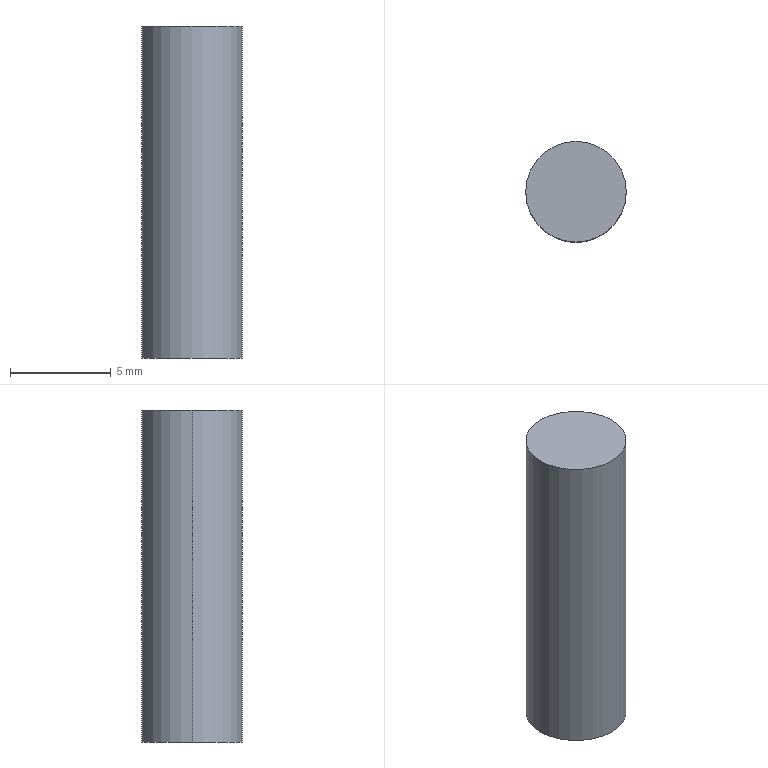Part | STEP file | Top bronze bushing custom screw SGN-2-26 | 1 solid | 11 faces | box 5 x 5 x 16.5 mm | volume 302.577 mm3 | plane 9 | cylinder 2 | commonest cylinder face diameters 5 x2
STEP:
#1=CARTESIAN_POINT('',(0.,0.,0.));
#2=DIRECTION('',(0.,0.,1.));
#3=DIRECTION('',(1.,0.,0.));
#4=AXIS2_PLACEMENT_3D('',#1,#2,#3);
#5=CARTESIAN_POINT('',(2.5,0.,16.5));
#6=VERTEX_POINT('',#5);
#7=CARTESIAN_POINT('',(-2.5,0.,16.5));
#8=VERTEX_POINT('',#7);
#9=CARTESIAN_POINT('',(0.,0.,16.5));
#10=DIRECTION('',(0.,0.,1.));
#11=DIRECTION('',(1.,0.,0.));
#12=AXIS2_PLACEMENT_3D('',#9,#10,#11);
#13=CIRCLE('',#12,2.5);
#14=CARTESIAN_POINT('',(0.,0.,16.5));
#15=DIRECTION('',(0.,0.,-1.));
#16=DIRECTION('',(-1.,0.,0.));
#17=AXIS2_PLACEMENT_3D('',#14,#15,#16);
#18=CYLINDRICAL_SURFACE('',#17,2.5);
#19=CARTESIAN_POINT('',(3.142,0.));
#20=DIRECTION('',(-1.,0.));
#21=VECTOR('',#20,1.);
#22=LINE('',#19,#21);
#23=(GEOMETRIC_REPRESENTATION_CONTEXT(2)PARAMETRIC_REPRESENTATION_CONTEXT()REPRESENTATION_CONTEXT('',''));
#24=DEFINITIONAL_REPRESENTATION('',(#22),#23);
#25=PCURVE('',#18,#24);
#26=CARTESIAN_POINT('',(0.,0.,16.5));
#27=DIRECTION('',(0.,0.,1.));
#28=DIRECTION('',(1.,0.,0.));
#29=AXIS2_PLACEMENT_3D('',#26,#27,#28);
#30=PLANE('',#29);
#31=CARTESIAN_POINT('',(0.,0.));
#32=DIRECTION('',(1.,0.));
#33=AXIS2_PLACEMENT_2D('',#31,#32);
#34=CIRCLE('',#33,2.5);
#35=(GEOMETRIC_REPRESENTATION_CONTEXT(2)PARAMETRIC_REPRESENTATION_CONTEXT()REPRESENTATION_CONTEXT('',''));
#36=DEFINITIONAL_REPRESENTATION('',(#34),#35);
#37=PCURVE('',#30,#36);
#38=SURFACE_CURVE('',#13,(#25,#37),.PCURVE_S1.);
#39=EDGE_CURVE('',#6,#8,#38,.T.);
#40=ORIENTED_EDGE('',*,*,#39,.F.);
#41=CARTESIAN_POINT('',(2.5,0.,0.));
#42=VERTEX_POINT('',#41);
#43=CARTESIAN_POINT('',(2.5,0.,16.5));
#44=DIRECTION('',(0.,0.,-1.));
#45=VECTOR('',#44,1.);
#46=LINE('',#43,#45);
#47=CARTESIAN_POINT('',(3.142,0.));
#48=DIRECTION('',(0.,1.));
#49=VECTOR('',#48,1.);
#50=LINE('',#47,#49);
#51=(GEOMETRIC_REPRESENTATION_CONTEXT(2)PARAMETRIC_REPRESENTATION_CONTEXT()REPRESENTATION_CONTEXT('',''));
#52=DEFINITIONAL_REPRESENTATION('',(#50),#51);
#53=PCURVE('',#18,#52);
#54=CARTESIAN_POINT('',(0.,0.,16.5));
#55=DIRECTION('',(0.,0.,-1.));
#56=DIRECTION('',(-1.,0.,0.));
#57=AXIS2_PLACEMENT_3D('',#54,#55,#56);
#58=CYLINDRICAL_SURFACE('',#57,2.5);
#59=CARTESIAN_POINT('',(3.142,0.));
#60=DIRECTION('',(0.,1.));
#61=VECTOR('',#60,1.);
#62=LINE('',#59,#61);
#63=(GEOMETRIC_REPRESENTATION_CONTEXT(2)PARAMETRIC_REPRESENTATION_CONTEXT()REPRESENTATION_CONTEXT('',''));
#64=DEFINITIONAL_REPRESENTATION('',(#62),#63);
#65=PCURVE('',#58,#64);
#66=SURFACE_CURVE('',#46,(#53,#65),.PCURVE_S1.);
#67=EDGE_CURVE('',#6,#42,#66,.T.);
#68=ORIENTED_EDGE('',*,*,#67,.T.);
#69=CARTESIAN_POINT('',(-2.5,0.,0.));
#70=VERTEX_POINT('',#69);
#71=CARTESIAN_POINT('',(0.,0.,0.));
#72=DIRECTION('',(0.,0.,1.));
#73=DIRECTION('',(1.,0.,0.));
#74=AXIS2_PLACEMENT_3D('',#71,#72,#73);
#75=CIRCLE('',#74,2.5);
#76=CARTESIAN_POINT('',(3.142,16.5));
#77=DIRECTION('',(-1.,0.));
#78=VECTOR('',#77,1.);
#79=LINE('',#76,#78);
#80=(GEOMETRIC_REPRESENTATION_CONTEXT(2)PARAMETRIC_REPRESENTATION_CONTEXT()REPRESENTATION_CONTEXT('',''));
#81=DEFINITIONAL_REPRESENTATION('',(#79),#80);
#82=PCURVE('',#18,#81);
#83=CARTESIAN_POINT('',(0.,0.,0.));
#84=DIRECTION('',(0.,0.,1.));
#85=DIRECTION('',(1.,0.,0.));
#86=AXIS2_PLACEMENT_3D('',#83,#84,#85);
#87=PLANE('',#86);
#88=CARTESIAN_POINT('',(0.,0.));
#89=DIRECTION('',(1.,0.));
#90=AXIS2_PLACEMENT_2D('',#88,#89);
#91=CIRCLE('',#90,2.5);
#92=(GEOMETRIC_REPRESENTATION_CONTEXT(2)PARAMETRIC_REPRESENTATION_CONTEXT()REPRESENTATION_CONTEXT('',''));
#93=DEFINITIONAL_REPRESENTATION('',(#91),#92);
#94=PCURVE('',#87,#93);
#95=SURFACE_CURVE('',#75,(#82,#94),.PCURVE_S1.);
#96=EDGE_CURVE('',#42,#70,#95,.T.);
#97=ORIENTED_EDGE('',*,*,#96,.T.);
#98=CARTESIAN_POINT('',(-2.5,0.,16.5));
#99=DIRECTION('',(0.,0.,-1.));
#100=VECTOR('',#99,1.);
#101=LINE('',#98,#100);
#102=CARTESIAN_POINT('',(0.,0.));
#103=DIRECTION('',(0.,1.));
#104=VECTOR('',#103,1.);
#105=LINE('',#102,#104);
#106=(GEOMETRIC_REPRESENTATION_CONTEXT(2)PARAMETRIC_REPRESENTATION_CONTEXT()REPRESENTATION_CONTEXT('',''));
#107=DEFINITIONAL_REPRESENTATION('',(#105),#106);
#108=PCURVE('',#18,#107);
#109=CARTESIAN_POINT('',(6.283,0.));
#110=DIRECTION('',(0.,1.));
#111=VECTOR('',#110,1.);
#112=LINE('',#109,#111);
#113=(GEOMETRIC_REPRESENTATION_CONTEXT(2)PARAMETRIC_REPRESENTATION_CONTEXT()REPRESENTATION_CONTEXT('',''));
#114=DEFINITIONAL_REPRESENTATION('',(#112),#113);
#115=PCURVE('',#58,#114);
#116=SURFACE_CURVE('',#101,(#108,#115),.PCURVE_S1.);
#117=EDGE_CURVE('',#8,#70,#116,.T.);
#118=ORIENTED_EDGE('',*,*,#117,.F.);
#119=EDGE_LOOP('',(#40,#68,#97,#118));
#120=FACE_BOUND('',#119,.T.);
#121=ADVANCED_FACE('',(#120),#18,.T.);
#122=ORIENTED_EDGE('',*,*,#67,.F.);
#123=CARTESIAN_POINT('',(0.,0.,16.5));
#124=DIRECTION('',(0.,0.,1.));
#125=DIRECTION('',(1.,0.,0.));
#126=AXIS2_PLACEMENT_3D('',#123,#124,#125);
#127=CIRCLE('',#126,2.5);
#128=CARTESIAN_POINT('',(9.425,0.));
#129=DIRECTION('',(-1.,0.));
#130=VECTOR('',#129,1.);
#131=LINE('',#128,#130);
#132=(GEOMETRIC_REPRESENTATION_CONTEXT(2)PARAMETRIC_REPRESENTATION_CONTEXT()REPRESENTATION_CONTEXT('',''));
#133=DEFINITIONAL_REPRESENTATION('',(#131),#132);
#134=PCURVE('',#58,#133);
#135=CARTESIAN_POINT('',(0.,0.));
#136=DIRECTION('',(1.,0.));
#137=AXIS2_PLACEMENT_2D('',#135,#136);
#138=CIRCLE('',#137,2.5);
#139=(GEOMETRIC_REPRESENTATION_CONTEXT(2)PARAMETRIC_REPRESENTATION_CONTEXT()REPRESENTATION_CONTEXT('',''));
#140=DEFINITIONAL_REPRESENTATION('',(#138),#139);
#141=PCURVE('',#30,#140);
#142=SURFACE_CURVE('',#127,(#134,#141),.PCURVE_S1.);
#143=EDGE_CURVE('',#8,#6,#142,.T.);
#144=ORIENTED_EDGE('',*,*,#143,.F.);
#145=ORIENTED_EDGE('',*,*,#117,.T.);
#146=CARTESIAN_POINT('',(0.,0.,0.));
#147=DIRECTION('',(0.,0.,1.));
#148=DIRECTION('',(1.,0.,0.));
#149=AXIS2_PLACEMENT_3D('',#146,#147,#148);
#150=CIRCLE('',#149,2.5);
#151=CARTESIAN_POINT('',(9.425,16.5));
#152=DIRECTION('',(-1.,0.));
#153=VECTOR('',#152,1.);
#154=LINE('',#151,#153);
#155=(GEOMETRIC_REPRESENTATION_CONTEXT(2)PARAMETRIC_REPRESENTATION_CONTEXT()REPRESENTATION_CONTEXT('',''));
#156=DEFINITIONAL_REPRESENTATION('',(#154),#155);
#157=PCURVE('',#58,#156);
#158=CARTESIAN_POINT('',(0.,0.));
#159=DIRECTION('',(1.,0.));
#160=AXIS2_PLACEMENT_2D('',#158,#159);
#161=CIRCLE('',#160,2.5);
#162=(GEOMETRIC_REPRESENTATION_CONTEXT(2)PARAMETRIC_REPRESENTATION_CONTEXT()REPRESENTATION_CONTEXT('',''));
#163=DEFINITIONAL_REPRESENTATION('',(#161),#162);
#164=PCURVE('',#87,#163);
#165=SURFACE_CURVE('',#150,(#157,#164),.PCURVE_S1.);
#166=EDGE_CURVE('',#70,#42,#165,.T.);
#167=ORIENTED_EDGE('',*,*,#166,.T.);
#168=EDGE_LOOP('',(#122,#144,#145,#167));
#169=FACE_BOUND('',#168,.T.);
#170=ADVANCED_FACE('',(#169),#58,.T.);
#171=ORIENTED_EDGE('',*,*,#143,.T.);
#172=ORIENTED_EDGE('',*,*,#39,.T.);
#173=EDGE_LOOP('',(#171,#172));
#174=FACE_BOUND('',#173,.T.);
#175=ADVANCED_FACE('',(#174),#30,.T.);
#176=CARTESIAN_POINT('',(0.,1.657,0.));
#177=VERTEX_POINT('',#176);
#178=CARTESIAN_POINT('',(1.435,0.8285,0.));
#179=VERTEX_POINT('',#178);
#180=CARTESIAN_POINT('',(0.,1.657,0.));
#181=DIRECTION('',(0.866,-0.5,0.));
#182=VECTOR('',#181,1.);
#183=LINE('',#180,#182);
#184=CARTESIAN_POINT('',(0.,1.657));
#185=DIRECTION('',(0.866,-0.5));
#186=VECTOR('',#185,1.);
#187=LINE('',#184,#186);
#188=(GEOMETRIC_REPRESENTATION_CONTEXT(2)PARAMETRIC_REPRESENTATION_CONTEXT()REPRESENTATION_CONTEXT('',''));
#189=DEFINITIONAL_REPRESENTATION('',(#187),#188);
#190=PCURVE('',#87,#189);
#191=CARTESIAN_POINT('',(0.,1.657,3.));
#192=DIRECTION('',(0.5,0.866,0.));
#193=DIRECTION('',(-0.866,0.5,0.));
#194=AXIS2_PLACEMENT_3D('',#191,#192,#193);
#195=PLANE('',#194);
#196=CARTESIAN_POINT('',(0.,-3.));
#197=DIRECTION('',(-1.,0.));
#198=VECTOR('',#197,1.);
#199=LINE('',#196,#198);
#200=(GEOMETRIC_REPRESENTATION_CONTEXT(2)PARAMETRIC_REPRESENTATION_CONTEXT()REPRESENTATION_CONTEXT('',''));
#201=DEFINITIONAL_REPRESENTATION('',(#199),#200);
#202=PCURVE('',#195,#201);
#203=SURFACE_CURVE('',#183,(#190,#202),.PCURVE_S1.);
#204=EDGE_CURVE('',#177,#179,#203,.T.);
#205=ORIENTED_EDGE('',*,*,#204,.F.);
#206=CARTESIAN_POINT('',(-1.435,0.8285,0.));
#207=VERTEX_POINT('',#206);
#208=CARTESIAN_POINT('',(-1.435,0.8285,0.));
#209=DIRECTION('',(0.866,0.5,0.));
#210=VECTOR('',#209,1.);
#211=LINE('',#208,#210);
#212=CARTESIAN_POINT('',(-1.435,0.8285));
#213=DIRECTION('',(0.866,0.5));
#214=VECTOR('',#213,1.);
#215=LINE('',#212,#214);
#216=(GEOMETRIC_REPRESENTATION_CONTEXT(2)PARAMETRIC_REPRESENTATION_CONTEXT()REPRESENTATION_CONTEXT('',''));
#217=DEFINITIONAL_REPRESENTATION('',(#215),#216);
#218=PCURVE('',#87,#217);
#219=CARTESIAN_POINT('',(-1.435,0.8285,3.));
#220=DIRECTION('',(-0.5,0.866,0.));
#221=DIRECTION('',(-0.866,-0.5,0.));
#222=AXIS2_PLACEMENT_3D('',#219,#220,#221);
#223=PLANE('',#222);
#224=CARTESIAN_POINT('',(0.,-3.));
#225=DIRECTION('',(-1.,0.));
#226=VECTOR('',#225,1.);
#227=LINE('',#224,#226);
#228=(GEOMETRIC_REPRESENTATION_CONTEXT(2)PARAMETRIC_REPRESENTATION_CONTEXT()REPRESENTATION_CONTEXT('',''));
#229=DEFINITIONAL_REPRESENTATION('',(#227),#228);
#230=PCURVE('',#223,#229);
#231=SURFACE_CURVE('',#211,(#218,#230),.PCURVE_S1.);
#232=EDGE_CURVE('',#207,#177,#231,.T.);
#233=ORIENTED_EDGE('',*,*,#232,.F.);
#234=CARTESIAN_POINT('',(-1.435,-0.8285,0.));
#235=VERTEX_POINT('',#234);
#236=CARTESIAN_POINT('',(-1.435,-0.8285,0.));
#237=DIRECTION('',(0.,1.,0.));
#238=VECTOR('',#237,1.);
#239=LINE('',#236,#238);
#240=CARTESIAN_POINT('',(-1.435,-0.8285));
#241=DIRECTION('',(0.,1.));
#242=VECTOR('',#241,1.);
#243=LINE('',#240,#242);
#244=(GEOMETRIC_REPRESENTATION_CONTEXT(2)PARAMETRIC_REPRESENTATION_CONTEXT()REPRESENTATION_CONTEXT('',''));
#245=DEFINITIONAL_REPRESENTATION('',(#243),#244);
#246=PCURVE('',#87,#245);
#247=CARTESIAN_POINT('',(-1.435,-0.8285,3.));
#248=DIRECTION('',(-1.,0.,0.));
#249=DIRECTION('',(0.,-1.,0.));
#250=AXIS2_PLACEMENT_3D('',#247,#248,#249);
#251=PLANE('',#250);
#252=CARTESIAN_POINT('',(0.,-3.));
#253=DIRECTION('',(-1.,0.));
#254=VECTOR('',#253,1.);
#255=LINE('',#252,#254);
#256=(GEOMETRIC_REPRESENTATION_CONTEXT(2)PARAMETRIC_REPRESENTATION_CONTEXT()REPRESENTATION_CONTEXT('',''));
#257=DEFINITIONAL_REPRESENTATION('',(#255),#256);
#258=PCURVE('',#251,#257);
#259=SURFACE_CURVE('',#239,(#246,#258),.PCURVE_S1.);
#260=EDGE_CURVE('',#235,#207,#259,.T.);
#261=ORIENTED_EDGE('',*,*,#260,.F.);
#262=CARTESIAN_POINT('',(0.,-1.657,0.));
#263=VERTEX_POINT('',#262);
#264=CARTESIAN_POINT('',(0.,-1.657,0.));
#265=DIRECTION('',(-0.866,0.5,0.));
#266=VECTOR('',#265,1.);
#267=LINE('',#264,#266);
#268=CARTESIAN_POINT('',(0.,-1.657));
#269=DIRECTION('',(-0.866,0.5));
#270=VECTOR('',#269,1.);
#271=LINE('',#268,#270);
#272=(GEOMETRIC_REPRESENTATION_CONTEXT(2)PARAMETRIC_REPRESENTATION_CONTEXT()REPRESENTATION_CONTEXT('',''));
#273=DEFINITIONAL_REPRESENTATION('',(#271),#272);
#274=PCURVE('',#87,#273);
#275=CARTESIAN_POINT('',(0.,-1.657,3.));
#276=DIRECTION('',(-0.5,-0.866,0.));
#277=DIRECTION('',(0.866,-0.5,0.));
#278=AXIS2_PLACEMENT_3D('',#275,#276,#277);
#279=PLANE('',#278);
#280=CARTESIAN_POINT('',(0.,-3.));
#281=DIRECTION('',(-1.,0.));
#282=VECTOR('',#281,1.);
#283=LINE('',#280,#282);
#284=(GEOMETRIC_REPRESENTATION_CONTEXT(2)PARAMETRIC_REPRESENTATION_CONTEXT()REPRESENTATION_CONTEXT('',''));
#285=DEFINITIONAL_REPRESENTATION('',(#283),#284);
#286=PCURVE('',#279,#285);
#287=SURFACE_CURVE('',#267,(#274,#286),.PCURVE_S1.);
#288=EDGE_CURVE('',#263,#235,#287,.T.);
#289=ORIENTED_EDGE('',*,*,#288,.F.);
#290=CARTESIAN_POINT('',(1.435,-0.8285,0.));
#291=VERTEX_POINT('',#290);
#292=CARTESIAN_POINT('',(1.435,-0.8285,0.));
#293=DIRECTION('',(-0.866,-0.5,0.));
#294=VECTOR('',#293,1.);
#295=LINE('',#292,#294);
#296=CARTESIAN_POINT('',(1.435,-0.8285));
#297=DIRECTION('',(-0.866,-0.5));
#298=VECTOR('',#297,1.);
#299=LINE('',#296,#298);
#300=(GEOMETRIC_REPRESENTATION_CONTEXT(2)PARAMETRIC_REPRESENTATION_CONTEXT()REPRESENTATION_CONTEXT('',''));
#301=DEFINITIONAL_REPRESENTATION('',(#299),#300);
#302=PCURVE('',#87,#301);
#303=CARTESIAN_POINT('',(1.435,-0.8285,3.));
#304=DIRECTION('',(0.5,-0.866,0.));
#305=DIRECTION('',(0.866,0.5,0.));
#306=AXIS2_PLACEMENT_3D('',#303,#304,#305);
#307=PLANE('',#306);
#308=CARTESIAN_POINT('',(0.,-3.));
#309=DIRECTION('',(-1.,0.));
#310=VECTOR('',#309,1.);
#311=LINE('',#308,#310);
#312=(GEOMETRIC_REPRESENTATION_CONTEXT(2)PARAMETRIC_REPRESENTATION_CONTEXT()REPRESENTATION_CONTEXT('',''));
#313=DEFINITIONAL_REPRESENTATION('',(#311),#312);
#314=PCURVE('',#307,#313);
#315=SURFACE_CURVE('',#295,(#302,#314),.PCURVE_S1.);
#316=EDGE_CURVE('',#291,#263,#315,.T.);
#317=ORIENTED_EDGE('',*,*,#316,.F.);
#318=CARTESIAN_POINT('',(1.435,0.8285,0.));
#319=DIRECTION('',(0.,-1.,0.));
#320=VECTOR('',#319,1.);
#321=LINE('',#318,#320);
#322=CARTESIAN_POINT('',(1.435,0.8285));
#323=DIRECTION('',(0.,-1.));
#324=VECTOR('',#323,1.);
#325=LINE('',#322,#324);
#326=(GEOMETRIC_REPRESENTATION_CONTEXT(2)PARAMETRIC_REPRESENTATION_CONTEXT()REPRESENTATION_CONTEXT('',''));
#327=DEFINITIONAL_REPRESENTATION('',(#325),#326);
#328=PCURVE('',#87,#327);
#329=CARTESIAN_POINT('',(1.435,0.8285,3.));
#330=DIRECTION('',(1.,0.,0.));
#331=DIRECTION('',(0.,1.,0.));
#332=AXIS2_PLACEMENT_3D('',#329,#330,#331);
#333=PLANE('',#332);
#334=CARTESIAN_POINT('',(0.,-3.));
#335=DIRECTION('',(-1.,0.));
#336=VECTOR('',#335,1.);
#337=LINE('',#334,#336);
#338=(GEOMETRIC_REPRESENTATION_CONTEXT(2)PARAMETRIC_REPRESENTATION_CONTEXT()REPRESENTATION_CONTEXT('',''));
#339=DEFINITIONAL_REPRESENTATION('',(#337),#338);
#340=PCURVE('',#333,#339);
#341=SURFACE_CURVE('',#321,(#328,#340),.PCURVE_S1.);
#342=EDGE_CURVE('',#179,#291,#341,.T.);
#343=ORIENTED_EDGE('',*,*,#342,.F.);
#344=EDGE_LOOP('',(#205,#233,#261,#289,#317,#343));
#345=FACE_BOUND('',#344,.T.);
#346=ORIENTED_EDGE('',*,*,#166,.F.);
#347=ORIENTED_EDGE('',*,*,#96,.F.);
#348=EDGE_LOOP('',(#346,#347));
#349=FACE_BOUND('',#348,.T.);
#350=ADVANCED_FACE('',(#345,#349),#87,.F.);
#351=ORIENTED_EDGE('',*,*,#232,.T.);
#352=CARTESIAN_POINT('',(0.,1.657,3.));
#353=VERTEX_POINT('',#352);
#354=CARTESIAN_POINT('',(0.,1.657,3.));
#355=DIRECTION('',(0.,0.,-1.));
#356=VECTOR('',#355,1.);
#357=LINE('',#354,#356);
#358=CARTESIAN_POINT('',(-1.657,0.));
#359=DIRECTION('',(0.,-1.));
#360=VECTOR('',#359,1.);
#361=LINE('',#358,#360);
#362=(GEOMETRIC_REPRESENTATION_CONTEXT(2)PARAMETRIC_REPRESENTATION_CONTEXT()REPRESENTATION_CONTEXT('',''));
#363=DEFINITIONAL_REPRESENTATION('',(#361),#362);
#364=PCURVE('',#223,#363);
#365=CARTESIAN_POINT('',(0.,0.));
#366=DIRECTION('',(0.,-1.));
#367=VECTOR('',#366,1.);
#368=LINE('',#365,#367);
#369=(GEOMETRIC_REPRESENTATION_CONTEXT(2)PARAMETRIC_REPRESENTATION_CONTEXT()REPRESENTATION_CONTEXT('',''));
#370=DEFINITIONAL_REPRESENTATION('',(#368),#369);
#371=PCURVE('',#195,#370);
#372=SURFACE_CURVE('',#357,(#364,#371),.PCURVE_S1.);
#373=EDGE_CURVE('',#353,#177,#372,.T.);
#374=ORIENTED_EDGE('',*,*,#373,.F.);
#375=CARTESIAN_POINT('',(-1.435,0.8285,3.));
#376=VERTEX_POINT('',#375);
#377=CARTESIAN_POINT('',(-1.435,0.8285,3.));
#378=DIRECTION('',(0.866,0.5,0.));
#379=VECTOR('',#378,1.);
#380=LINE('',#377,#379);
#381=CARTESIAN_POINT('',(0.,0.));
#382=DIRECTION('',(-1.,0.));
#383=VECTOR('',#382,1.);
#384=LINE('',#381,#383);
#385=(GEOMETRIC_REPRESENTATION_CONTEXT(2)PARAMETRIC_REPRESENTATION_CONTEXT()REPRESENTATION_CONTEXT('',''));
#386=DEFINITIONAL_REPRESENTATION('',(#384),#385);
#387=PCURVE('',#223,#386);
#388=CARTESIAN_POINT('',(0.,0.,3.));
#389=DIRECTION('',(0.,0.,-1.));
#390=DIRECTION('',(-1.,0.,0.));
#391=AXIS2_PLACEMENT_3D('',#388,#389,#390);
#392=PLANE('',#391);
#393=CARTESIAN_POINT('',(1.435,0.8285));
#394=DIRECTION('',(-0.866,0.5));
#395=VECTOR('',#394,1.);
#396=LINE('',#393,#395);
#397=(GEOMETRIC_REPRESENTATION_CONTEXT(2)PARAMETRIC_REPRESENTATION_CONTEXT()REPRESENTATION_CONTEXT('',''));
#398=DEFINITIONAL_REPRESENTATION('',(#396),#397);
#399=PCURVE('',#392,#398);
#400=SURFACE_CURVE('',#380,(#387,#399),.PCURVE_S1.);
#401=EDGE_CURVE('',#376,#353,#400,.T.);
#402=ORIENTED_EDGE('',*,*,#401,.F.);
#403=CARTESIAN_POINT('',(-1.435,0.8285,3.));
#404=DIRECTION('',(0.,0.,-1.));
#405=VECTOR('',#404,1.);
#406=LINE('',#403,#405);
#407=CARTESIAN_POINT('',(0.,0.));
#408=DIRECTION('',(0.,-1.));
#409=VECTOR('',#408,1.);
#410=LINE('',#407,#409);
#411=(GEOMETRIC_REPRESENTATION_CONTEXT(2)PARAMETRIC_REPRESENTATION_CONTEXT()REPRESENTATION_CONTEXT('',''));
#412=DEFINITIONAL_REPRESENTATION('',(#410),#411);
#413=PCURVE('',#223,#412);
#414=CARTESIAN_POINT('',(-1.657,0.));
#415=DIRECTION('',(0.,-1.));
#416=VECTOR('',#415,1.);
#417=LINE('',#414,#416);
#418=(GEOMETRIC_REPRESENTATION_CONTEXT(2)PARAMETRIC_REPRESENTATION_CONTEXT()REPRESENTATION_CONTEXT('',''));
#419=DEFINITIONAL_REPRESENTATION('',(#417),#418);
#420=PCURVE('',#251,#419);
#421=SURFACE_CURVE('',#406,(#413,#420),.PCURVE_S1.);
#422=EDGE_CURVE('',#376,#207,#421,.T.);
#423=ORIENTED_EDGE('',*,*,#422,.T.);
#424=EDGE_LOOP('',(#351,#374,#402,#423));
#425=FACE_BOUND('',#424,.T.);
#426=ADVANCED_FACE('',(#425),#223,.F.);
#427=ORIENTED_EDGE('',*,*,#260,.T.);
#428=ORIENTED_EDGE('',*,*,#422,.F.);
#429=CARTESIAN_POINT('',(-1.435,-0.8285,3.));
#430=VERTEX_POINT('',#429);
#431=CARTESIAN_POINT('',(-1.435,-0.8285,3.));
#432=DIRECTION('',(0.,1.,0.));
#433=VECTOR('',#432,1.);
#434=LINE('',#431,#433);
#435=CARTESIAN_POINT('',(0.,0.));
#436=DIRECTION('',(-1.,0.));
#437=VECTOR('',#436,1.);
#438=LINE('',#435,#437);
#439=(GEOMETRIC_REPRESENTATION_CONTEXT(2)PARAMETRIC_REPRESENTATION_CONTEXT()REPRESENTATION_CONTEXT('',''));
#440=DEFINITIONAL_REPRESENTATION('',(#438),#439);
#441=PCURVE('',#251,#440);
#442=CARTESIAN_POINT('',(1.435,-0.8285));
#443=DIRECTION('',(0.,1.));
#444=VECTOR('',#443,1.);
#445=LINE('',#442,#444);
#446=(GEOMETRIC_REPRESENTATION_CONTEXT(2)PARAMETRIC_REPRESENTATION_CONTEXT()REPRESENTATION_CONTEXT('',''));
#447=DEFINITIONAL_REPRESENTATION('',(#445),#446);
#448=PCURVE('',#392,#447);
#449=SURFACE_CURVE('',#434,(#441,#448),.PCURVE_S1.);
#450=EDGE_CURVE('',#430,#376,#449,.T.);
#451=ORIENTED_EDGE('',*,*,#450,.F.);
#452=CARTESIAN_POINT('',(-1.435,-0.8285,3.));
#453=DIRECTION('',(0.,0.,-1.));
#454=VECTOR('',#453,1.);
#455=LINE('',#452,#454);
#456=CARTESIAN_POINT('',(0.,0.));
#457=DIRECTION('',(0.,-1.));
#458=VECTOR('',#457,1.);
#459=LINE('',#456,#458);
#460=(GEOMETRIC_REPRESENTATION_CONTEXT(2)PARAMETRIC_REPRESENTATION_CONTEXT()REPRESENTATION_CONTEXT('',''));
#461=DEFINITIONAL_REPRESENTATION('',(#459),#460);
#462=PCURVE('',#251,#461);
#463=CARTESIAN_POINT('',(-1.657,0.));
#464=DIRECTION('',(0.,-1.));
#465=VECTOR('',#464,1.);
#466=LINE('',#463,#465);
#467=(GEOMETRIC_REPRESENTATION_CONTEXT(2)PARAMETRIC_REPRESENTATION_CONTEXT()REPRESENTATION_CONTEXT('',''));
#468=DEFINITIONAL_REPRESENTATION('',(#466),#467);
#469=PCURVE('',#279,#468);
#470=SURFACE_CURVE('',#455,(#462,#469),.PCURVE_S1.);
#471=EDGE_CURVE('',#430,#235,#470,.T.);
#472=ORIENTED_EDGE('',*,*,#471,.T.);
#473=EDGE_LOOP('',(#427,#428,#451,#472));
#474=FACE_BOUND('',#473,.T.);
#475=ADVANCED_FACE('',(#474),#251,.F.);
#476=ORIENTED_EDGE('',*,*,#288,.T.);
#477=ORIENTED_EDGE('',*,*,#471,.F.);
#478=CARTESIAN_POINT('',(0.,-1.657,3.));
#479=VERTEX_POINT('',#478);
#480=CARTESIAN_POINT('',(0.,-1.657,3.));
#481=DIRECTION('',(-0.866,0.5,0.));
#482=VECTOR('',#481,1.);
#483=LINE('',#480,#482);
#484=CARTESIAN_POINT('',(0.,0.));
#485=DIRECTION('',(-1.,0.));
#486=VECTOR('',#485,1.);
#487=LINE('',#484,#486);
#488=(GEOMETRIC_REPRESENTATION_CONTEXT(2)PARAMETRIC_REPRESENTATION_CONTEXT()REPRESENTATION_CONTEXT('',''));
#489=DEFINITIONAL_REPRESENTATION('',(#487),#488);
#490=PCURVE('',#279,#489);
#491=CARTESIAN_POINT('',(0.,-1.657));
#492=DIRECTION('',(0.866,0.5));
#493=VECTOR('',#492,1.);
#494=LINE('',#491,#493);
#495=(GEOMETRIC_REPRESENTATION_CONTEXT(2)PARAMETRIC_REPRESENTATION_CONTEXT()REPRESENTATION_CONTEXT('',''));
#496=DEFINITIONAL_REPRESENTATION('',(#494),#495);
#497=PCURVE('',#392,#496);
#498=SURFACE_CURVE('',#483,(#490,#497),.PCURVE_S1.);
#499=EDGE_CURVE('',#479,#430,#498,.T.);
#500=ORIENTED_EDGE('',*,*,#499,.F.);
#501=CARTESIAN_POINT('',(0.,-1.657,3.));
#502=DIRECTION('',(0.,0.,-1.));
#503=VECTOR('',#502,1.);
#504=LINE('',#501,#503);
#505=CARTESIAN_POINT('',(0.,0.));
#506=DIRECTION('',(0.,-1.));
#507=VECTOR('',#506,1.);
#508=LINE('',#505,#507);
#509=(GEOMETRIC_REPRESENTATION_CONTEXT(2)PARAMETRIC_REPRESENTATION_CONTEXT()REPRESENTATION_CONTEXT('',''));
#510=DEFINITIONAL_REPRESENTATION('',(#508),#509);
#511=PCURVE('',#279,#510);
#512=CARTESIAN_POINT('',(-1.657,0.));
#513=DIRECTION('',(0.,-1.));
#514=VECTOR('',#513,1.);
#515=LINE('',#512,#514);
#516=(GEOMETRIC_REPRESENTATION_CONTEXT(2)PARAMETRIC_REPRESENTATION_CONTEXT()REPRESENTATION_CONTEXT('',''));
#517=DEFINITIONAL_REPRESENTATION('',(#515),#516);
#518=PCURVE('',#307,#517);
#519=SURFACE_CURVE('',#504,(#511,#518),.PCURVE_S1.);
#520=EDGE_CURVE('',#479,#263,#519,.T.);
#521=ORIENTED_EDGE('',*,*,#520,.T.);
#522=EDGE_LOOP('',(#476,#477,#500,#521));
#523=FACE_BOUND('',#522,.T.);
#524=ADVANCED_FACE('',(#523),#279,.F.);
#525=ORIENTED_EDGE('',*,*,#316,.T.);
#526=ORIENTED_EDGE('',*,*,#520,.F.);
#527=CARTESIAN_POINT('',(1.435,-0.8285,3.));
#528=VERTEX_POINT('',#527);
#529=CARTESIAN_POINT('',(1.435,-0.8285,3.));
#530=DIRECTION('',(-0.866,-0.5,0.));
#531=VECTOR('',#530,1.);
#532=LINE('',#529,#531);
#533=CARTESIAN_POINT('',(0.,0.));
#534=DIRECTION('',(-1.,0.));
#535=VECTOR('',#534,1.);
#536=LINE('',#533,#535);
#537=(GEOMETRIC_REPRESENTATION_CONTEXT(2)PARAMETRIC_REPRESENTATION_CONTEXT()REPRESENTATION_CONTEXT('',''));
#538=DEFINITIONAL_REPRESENTATION('',(#536),#537);
#539=PCURVE('',#307,#538);
#540=CARTESIAN_POINT('',(-1.435,-0.8285));
#541=DIRECTION('',(0.866,-0.5));
#542=VECTOR('',#541,1.);
#543=LINE('',#540,#542);
#544=(GEOMETRIC_REPRESENTATION_CONTEXT(2)PARAMETRIC_REPRESENTATION_CONTEXT()REPRESENTATION_CONTEXT('',''));
#545=DEFINITIONAL_REPRESENTATION('',(#543),#544);
#546=PCURVE('',#392,#545);
#547=SURFACE_CURVE('',#532,(#539,#546),.PCURVE_S1.);
#548=EDGE_CURVE('',#528,#479,#547,.T.);
#549=ORIENTED_EDGE('',*,*,#548,.F.);
#550=CARTESIAN_POINT('',(1.435,-0.8285,3.));
#551=DIRECTION('',(0.,0.,-1.));
#552=VECTOR('',#551,1.);
#553=LINE('',#550,#552);
#554=CARTESIAN_POINT('',(0.,0.));
#555=DIRECTION('',(0.,-1.));
#556=VECTOR('',#555,1.);
#557=LINE('',#554,#556);
#558=(GEOMETRIC_REPRESENTATION_CONTEXT(2)PARAMETRIC_REPRESENTATION_CONTEXT()REPRESENTATION_CONTEXT('',''));
#559=DEFINITIONAL_REPRESENTATION('',(#557),#558);
#560=PCURVE('',#307,#559);
#561=CARTESIAN_POINT('',(-1.657,0.));
#562=DIRECTION('',(0.,-1.));
#563=VECTOR('',#562,1.);
#564=LINE('',#561,#563);
#565=(GEOMETRIC_REPRESENTATION_CONTEXT(2)PARAMETRIC_REPRESENTATION_CONTEXT()REPRESENTATION_CONTEXT('',''));
#566=DEFINITIONAL_REPRESENTATION('',(#564),#565);
#567=PCURVE('',#333,#566);
#568=SURFACE_CURVE('',#553,(#560,#567),.PCURVE_S1.);
#569=EDGE_CURVE('',#528,#291,#568,.T.);
#570=ORIENTED_EDGE('',*,*,#569,.T.);
#571=EDGE_LOOP('',(#525,#526,#549,#570));
#572=FACE_BOUND('',#571,.T.);
#573=ADVANCED_FACE('',(#572),#307,.F.);
#574=ORIENTED_EDGE('',*,*,#342,.T.);
#575=ORIENTED_EDGE('',*,*,#569,.F.);
#576=CARTESIAN_POINT('',(1.435,0.8285,3.));
#577=VERTEX_POINT('',#576);
#578=CARTESIAN_POINT('',(1.435,0.8285,3.));
#579=DIRECTION('',(0.,-1.,0.));
#580=VECTOR('',#579,1.);
#581=LINE('',#578,#580);
#582=CARTESIAN_POINT('',(0.,0.));
#583=DIRECTION('',(-1.,0.));
#584=VECTOR('',#583,1.);
#585=LINE('',#582,#584);
#586=(GEOMETRIC_REPRESENTATION_CONTEXT(2)PARAMETRIC_REPRESENTATION_CONTEXT()REPRESENTATION_CONTEXT('',''));
#587=DEFINITIONAL_REPRESENTATION('',(#585),#586);
#588=PCURVE('',#333,#587);
#589=CARTESIAN_POINT('',(-1.435,0.8285));
#590=DIRECTION('',(0.,-1.));
#591=VECTOR('',#590,1.);
#592=LINE('',#589,#591);
#593=(GEOMETRIC_REPRESENTATION_CONTEXT(2)PARAMETRIC_REPRESENTATION_CONTEXT()REPRESENTATION_CONTEXT('',''));
#594=DEFINITIONAL_REPRESENTATION('',(#592),#593);
#595=PCURVE('',#392,#594);
#596=SURFACE_CURVE('',#581,(#588,#595),.PCURVE_S1.);
#597=EDGE_CURVE('',#577,#528,#596,.T.);
#598=ORIENTED_EDGE('',*,*,#597,.F.);
#599=CARTESIAN_POINT('',(1.435,0.8285,3.));
#600=DIRECTION('',(0.,0.,-1.));
#601=VECTOR('',#600,1.);
#602=LINE('',#599,#601);
#603=CARTESIAN_POINT('',(0.,0.));
#604=DIRECTION('',(0.,-1.));
#605=VECTOR('',#604,1.);
#606=LINE('',#603,#605);
#607=(GEOMETRIC_REPRESENTATION_CONTEXT(2)PARAMETRIC_REPRESENTATION_CONTEXT()REPRESENTATION_CONTEXT('',''));
#608=DEFINITIONAL_REPRESENTATION('',(#606),#607);
#609=PCURVE('',#333,#608);
#610=CARTESIAN_POINT('',(-1.657,0.));
#611=DIRECTION('',(0.,-1.));
#612=VECTOR('',#611,1.);
#613=LINE('',#610,#612);
#614=(GEOMETRIC_REPRESENTATION_CONTEXT(2)PARAMETRIC_REPRESENTATION_CONTEXT()REPRESENTATION_CONTEXT('',''));
#615=DEFINITIONAL_REPRESENTATION('',(#613),#614);
#616=PCURVE('',#195,#615);
#617=SURFACE_CURVE('',#602,(#609,#616),.PCURVE_S1.);
#618=EDGE_CURVE('',#577,#179,#617,.T.);
#619=ORIENTED_EDGE('',*,*,#618,.T.);
#620=EDGE_LOOP('',(#574,#575,#598,#619));
#621=FACE_BOUND('',#620,.T.);
#622=ADVANCED_FACE('',(#621),#333,.F.);
#623=ORIENTED_EDGE('',*,*,#204,.T.);
#624=ORIENTED_EDGE('',*,*,#618,.F.);
#625=CARTESIAN_POINT('',(0.,1.657,3.));
#626=DIRECTION('',(0.866,-0.5,0.));
#627=VECTOR('',#626,1.);
#628=LINE('',#625,#627);
#629=CARTESIAN_POINT('',(0.,0.));
#630=DIRECTION('',(-1.,0.));
#631=VECTOR('',#630,1.);
#632=LINE('',#629,#631);
#633=(GEOMETRIC_REPRESENTATION_CONTEXT(2)PARAMETRIC_REPRESENTATION_CONTEXT()REPRESENTATION_CONTEXT('',''));
#634=DEFINITIONAL_REPRESENTATION('',(#632),#633);
#635=PCURVE('',#195,#634);
#636=CARTESIAN_POINT('',(0.,1.657));
#637=DIRECTION('',(-0.866,-0.5));
#638=VECTOR('',#637,1.);
#639=LINE('',#636,#638);
#640=(GEOMETRIC_REPRESENTATION_CONTEXT(2)PARAMETRIC_REPRESENTATION_CONTEXT()REPRESENTATION_CONTEXT('',''));
#641=DEFINITIONAL_REPRESENTATION('',(#639),#640);
#642=PCURVE('',#392,#641);
#643=SURFACE_CURVE('',#628,(#635,#642),.PCURVE_S1.);
#644=EDGE_CURVE('',#353,#577,#643,.T.);
#645=ORIENTED_EDGE('',*,*,#644,.F.);
#646=ORIENTED_EDGE('',*,*,#373,.T.);
#647=EDGE_LOOP('',(#623,#624,#645,#646));
#648=FACE_BOUND('',#647,.T.);
#649=ADVANCED_FACE('',(#648),#195,.F.);
#650=ORIENTED_EDGE('',*,*,#401,.T.);
#651=ORIENTED_EDGE('',*,*,#644,.T.);
#652=ORIENTED_EDGE('',*,*,#597,.T.);
#653=ORIENTED_EDGE('',*,*,#548,.T.);
#654=ORIENTED_EDGE('',*,*,#499,.T.);
#655=ORIENTED_EDGE('',*,*,#450,.T.);
#656=EDGE_LOOP('',(#650,#651,#652,#653,#654,#655));
#657=FACE_BOUND('',#656,.T.);
#658=ADVANCED_FACE('',(#657),#392,.T.);
#659=CLOSED_SHELL('',(#121,#170,#175,#350,#426,#475,#524,#573,#622,#649,#658));
#660=MANIFOLD_SOLID_BREP('',#659);
#661=(LENGTH_UNIT()NAMED_UNIT(*)SI_UNIT(.MILLI.,.METRE.));
#662=UNCERTAINTY_MEASURE_WITH_UNIT(LENGTH_MEASURE(0.0000001),#661,'','');
#663=(NAMED_UNIT(*)PLANE_ANGLE_UNIT()SI_UNIT($,.RADIAN.));
#664=(NAMED_UNIT(*)SI_UNIT($,.STERADIAN.)SOLID_ANGLE_UNIT());
#665=(GEOMETRIC_REPRESENTATION_CONTEXT(3)GLOBAL_UNCERTAINTY_ASSIGNED_CONTEXT((#662))GLOBAL_UNIT_ASSIGNED_CONTEXT((#661,#663,#664))REPRESENTATION_CONTEXT('',''));
#666=ADVANCED_BREP_SHAPE_REPRESENTATION('',(#4,#660),#665);